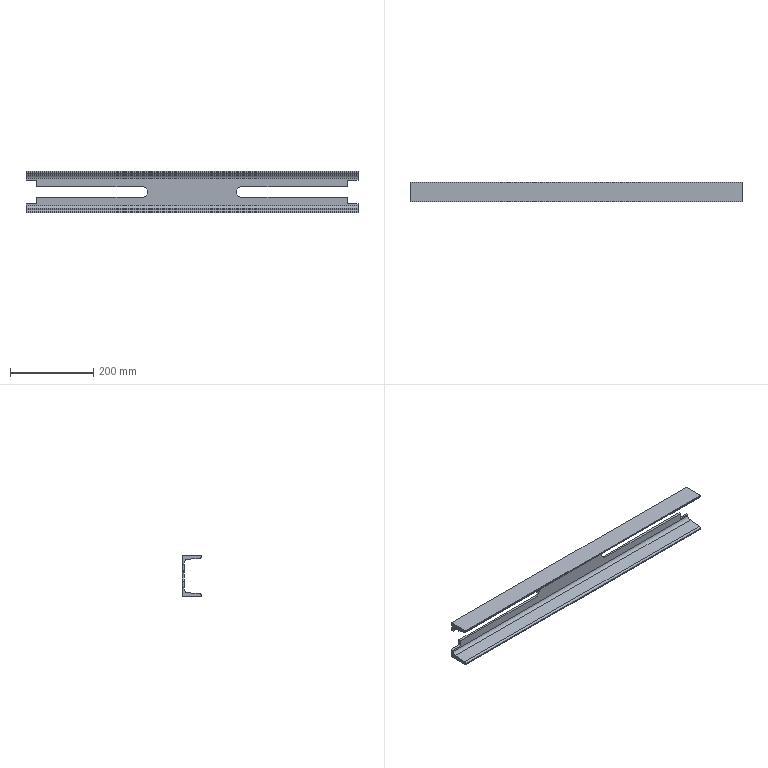Part | SolidWorks | features ICE 2, MirrorPattern 1, WeldMemberFeat 1, WeldmentFeature 1 | 1 solid | 30 faces | box 800 x 48 x 100 mm | volume 931477 mm3 | plane 24 | cylinder 6 | commonest cylinder face diameters 8.5 x2 17 x2 26 x2
STEP:
#1=CARTESIAN_POINT('',(400.,0.,78.));
#2=VERTEX_POINT('',#1);
#3=CARTESIAN_POINT('',(375.,0.,78.));
#4=VERTEX_POINT('',#3);
#5=CARTESIAN_POINT('',(400.,0.,78.));
#6=DIRECTION('',(-1.,0.,0.));
#7=VECTOR('',#6,1000.);
#8=LINE('',#5,#7);
#9=EDGE_CURVE('',#2,#4,#8,.T.);
#10=ORIENTED_EDGE('',*,*,#9,.T.);
#11=CARTESIAN_POINT('',(375.,0.,63.));
#12=VERTEX_POINT('',#11);
#13=CARTESIAN_POINT('',(375.,0.,78.));
#14=DIRECTION('',(0.,0.,-1.));
#15=VECTOR('',#14,1000.);
#16=LINE('',#13,#15);
#17=EDGE_CURVE('',#4,#12,#16,.T.);
#18=ORIENTED_EDGE('',*,*,#17,.T.);
#19=CARTESIAN_POINT('',(120.,0.,63.));
#20=VERTEX_POINT('',#19);
#21=CARTESIAN_POINT('',(680.,0.,63.));
#22=DIRECTION('',(-1.,0.,0.));
#23=VECTOR('',#22,1000.);
#24=LINE('',#21,#23);
#25=EDGE_CURVE('',#12,#20,#24,.T.);
#26=ORIENTED_EDGE('',*,*,#25,.T.);
#27=CARTESIAN_POINT('',(120.,0.,37.));
#28=VERTEX_POINT('',#27);
#29=CARTESIAN_POINT('',(120.,0.,50.));
#30=DIRECTION('',(0.,-1.,0.));
#31=DIRECTION('',(0.,0.,1.));
#32=AXIS2_PLACEMENT_3D('',#29,#30,#31);
#33=CIRCLE('',#32,13.);
#34=EDGE_CURVE('',#20,#28,#33,.T.);
#35=ORIENTED_EDGE('',*,*,#34,.T.);
#36=CARTESIAN_POINT('',(375.,0.,37.));
#37=VERTEX_POINT('',#36);
#38=CARTESIAN_POINT('',(680.,0.,37.));
#39=DIRECTION('',(1.,0.,0.));
#40=VECTOR('',#39,1000.);
#41=LINE('',#38,#40);
#42=EDGE_CURVE('',#28,#37,#41,.T.);
#43=ORIENTED_EDGE('',*,*,#42,.T.);
#44=CARTESIAN_POINT('',(375.,0.,22.));
#45=VERTEX_POINT('',#44);
#46=CARTESIAN_POINT('',(375.,0.,22.));
#47=DIRECTION('',(0.,0.,-1.));
#48=VECTOR('',#47,1000.);
#49=LINE('',#46,#48);
#50=EDGE_CURVE('',#37,#45,#49,.T.);
#51=ORIENTED_EDGE('',*,*,#50,.T.);
#52=CARTESIAN_POINT('',(400.,0.,22.));
#53=VERTEX_POINT('',#52);
#54=CARTESIAN_POINT('',(400.,0.,22.));
#55=DIRECTION('',(1.,0.,0.));
#56=VECTOR('',#55,1000.);
#57=LINE('',#54,#56);
#58=EDGE_CURVE('',#45,#53,#57,.T.);
#59=ORIENTED_EDGE('',*,*,#58,.T.);
#60=CARTESIAN_POINT('',(400.,0.,0.));
#61=VERTEX_POINT('',#60);
#62=CARTESIAN_POINT('',(400.,0.,100.));
#63=DIRECTION('',(0.,0.,-1.));
#64=VECTOR('',#63,1000.);
#65=LINE('',#62,#64);
#66=EDGE_CURVE('',#53,#61,#65,.T.);
#67=ORIENTED_EDGE('',*,*,#66,.T.);
#68=CARTESIAN_POINT('',(-400.,0.,0.));
#69=VERTEX_POINT('',#68);
#70=CARTESIAN_POINT('',(-400.,0.,0.));
#71=DIRECTION('',(1.,0.,0.));
#72=VECTOR('',#71,1000.);
#73=LINE('',#70,#72);
#74=EDGE_CURVE('',#69,#61,#73,.T.);
#75=ORIENTED_EDGE('',*,*,#74,.F.);
#76=CARTESIAN_POINT('',(-400.,0.,22.));
#77=VERTEX_POINT('',#76);
#78=CARTESIAN_POINT('',(-400.,0.,100.));
#79=DIRECTION('',(0.,0.,-1.));
#80=VECTOR('',#79,1000.);
#81=LINE('',#78,#80);
#82=EDGE_CURVE('',#77,#69,#81,.T.);
#83=ORIENTED_EDGE('',*,*,#82,.F.);
#84=CARTESIAN_POINT('',(-375.,0.,22.));
#85=VERTEX_POINT('',#84);
#86=CARTESIAN_POINT('',(-400.,0.,22.));
#87=DIRECTION('',(-1.,0.,0.));
#88=VECTOR('',#87,1000.);
#89=LINE('',#86,#88);
#90=EDGE_CURVE('',#85,#77,#89,.T.);
#91=ORIENTED_EDGE('',*,*,#90,.F.);
#92=CARTESIAN_POINT('',(-375.,0.,37.));
#93=VERTEX_POINT('',#92);
#94=CARTESIAN_POINT('',(-375.,0.,22.));
#95=DIRECTION('',(0.,0.,-1.));
#96=VECTOR('',#95,1000.);
#97=LINE('',#94,#96);
#98=EDGE_CURVE('',#93,#85,#97,.T.);
#99=ORIENTED_EDGE('',*,*,#98,.F.);
#100=CARTESIAN_POINT('',(-120.,0.,37.));
#101=VERTEX_POINT('',#100);
#102=CARTESIAN_POINT('',(-680.,0.,37.));
#103=DIRECTION('',(-1.,0.,0.));
#104=VECTOR('',#103,1000.);
#105=LINE('',#102,#104);
#106=EDGE_CURVE('',#101,#93,#105,.T.);
#107=ORIENTED_EDGE('',*,*,#106,.F.);
#108=CARTESIAN_POINT('',(-120.,0.,63.));
#109=VERTEX_POINT('',#108);
#110=CARTESIAN_POINT('',(-120.,0.,50.));
#111=DIRECTION('',(0.,1.,0.));
#112=DIRECTION('',(0.,0.,1.));
#113=AXIS2_PLACEMENT_3D('',#110,#111,#112);
#114=CIRCLE('',#113,13.);
#115=EDGE_CURVE('',#109,#101,#114,.T.);
#116=ORIENTED_EDGE('',*,*,#115,.F.);
#117=CARTESIAN_POINT('',(-375.,0.,63.));
#118=VERTEX_POINT('',#117);
#119=CARTESIAN_POINT('',(-680.,0.,63.));
#120=DIRECTION('',(1.,0.,0.));
#121=VECTOR('',#120,1000.);
#122=LINE('',#119,#121);
#123=EDGE_CURVE('',#118,#109,#122,.T.);
#124=ORIENTED_EDGE('',*,*,#123,.F.);
#125=CARTESIAN_POINT('',(-375.,0.,78.));
#126=VERTEX_POINT('',#125);
#127=CARTESIAN_POINT('',(-375.,0.,78.));
#128=DIRECTION('',(0.,0.,-1.));
#129=VECTOR('',#128,1000.);
#130=LINE('',#127,#129);
#131=EDGE_CURVE('',#126,#118,#130,.T.);
#132=ORIENTED_EDGE('',*,*,#131,.F.);
#133=CARTESIAN_POINT('',(-400.,0.,78.));
#134=VERTEX_POINT('',#133);
#135=CARTESIAN_POINT('',(-400.,0.,78.));
#136=DIRECTION('',(1.,0.,0.));
#137=VECTOR('',#136,1000.);
#138=LINE('',#135,#137);
#139=EDGE_CURVE('',#134,#126,#138,.T.);
#140=ORIENTED_EDGE('',*,*,#139,.F.);
#141=CARTESIAN_POINT('',(-400.,0.,100.));
#142=VERTEX_POINT('',#141);
#143=CARTESIAN_POINT('',(-400.,0.,100.));
#144=DIRECTION('',(0.,0.,-1.));
#145=VECTOR('',#144,1000.);
#146=LINE('',#143,#145);
#147=EDGE_CURVE('',#142,#134,#146,.T.);
#148=ORIENTED_EDGE('',*,*,#147,.F.);
#149=CARTESIAN_POINT('',(400.,0.,100.));
#150=VERTEX_POINT('',#149);
#151=CARTESIAN_POINT('',(-400.,0.,100.));
#152=DIRECTION('',(1.,0.,0.));
#153=VECTOR('',#152,1000.);
#154=LINE('',#151,#153);
#155=EDGE_CURVE('',#142,#150,#154,.T.);
#156=ORIENTED_EDGE('',*,*,#155,.T.);
#157=CARTESIAN_POINT('',(400.,0.,100.));
#158=DIRECTION('',(0.,0.,-1.));
#159=VECTOR('',#158,1000.);
#160=LINE('',#157,#159);
#161=EDGE_CURVE('',#150,#2,#160,.T.);
#162=ORIENTED_EDGE('',*,*,#161,.T.);
#163=EDGE_LOOP('',(#10,#18,#26,#35,#43,#51,#59,#67,#75,#83,#91,#99,#107,#116,#124,#132,#140,#148,#156,#162));
#164=FACE_OUTER_BOUND('',#163,.T.);
#165=CARTESIAN_POINT('',(-400.,0.,100.));
#166=DIRECTION('',(0.,-1.,0.));
#167=DIRECTION('',(1.,0.,0.));
#168=AXIS2_PLACEMENT_3D('',#165,#166,#167);
#169=PLANE('',#168);
#170=ADVANCED_FACE('',(#164),#169,.F.);
#171=CARTESIAN_POINT('',(400.,-5.3,78.));
#172=VERTEX_POINT('',#171);
#173=CARTESIAN_POINT('',(375.,-5.3,78.));
#174=VERTEX_POINT('',#173);
#175=CARTESIAN_POINT('',(-400.,-5.3,78.));
#176=DIRECTION('',(-1.,0.,0.));
#177=VECTOR('',#176,1000.);
#178=LINE('',#175,#177);
#179=EDGE_CURVE('',#172,#174,#178,.T.);
#180=ORIENTED_EDGE('',*,*,#179,.F.);
#181=CARTESIAN_POINT('',(400.,-5.3,81.673));
#182=VERTEX_POINT('',#181);
#183=CARTESIAN_POINT('',(400.,-5.3,81.673));
#184=DIRECTION('',(0.,0.,1.));
#185=VECTOR('',#184,1000.);
#186=LINE('',#183,#185);
#187=EDGE_CURVE('',#172,#182,#186,.T.);
#188=ORIENTED_EDGE('',*,*,#187,.T.);
#189=CARTESIAN_POINT('',(-400.,-5.3,81.673));
#190=VERTEX_POINT('',#189);
#191=CARTESIAN_POINT('',(-400.,-5.3,81.673));
#192=DIRECTION('',(1.,0.,0.));
#193=VECTOR('',#192,1000.);
#194=LINE('',#191,#193);
#195=EDGE_CURVE('',#190,#182,#194,.T.);
#196=ORIENTED_EDGE('',*,*,#195,.F.);
#197=CARTESIAN_POINT('',(-400.,-5.3,78.));
#198=VERTEX_POINT('',#197);
#199=CARTESIAN_POINT('',(-400.,-5.3,81.673));
#200=DIRECTION('',(0.,0.,1.));
#201=VECTOR('',#200,1000.);
#202=LINE('',#199,#201);
#203=EDGE_CURVE('',#198,#190,#202,.T.);
#204=ORIENTED_EDGE('',*,*,#203,.F.);
#205=CARTESIAN_POINT('',(-375.,-5.3,78.));
#206=VERTEX_POINT('',#205);
#207=CARTESIAN_POINT('',(-400.,-5.3,78.));
#208=DIRECTION('',(1.,0.,0.));
#209=VECTOR('',#208,1000.);
#210=LINE('',#207,#209);
#211=EDGE_CURVE('',#198,#206,#210,.T.);
#212=ORIENTED_EDGE('',*,*,#211,.T.);
#213=CARTESIAN_POINT('',(-375.,-5.3,63.));
#214=VERTEX_POINT('',#213);
#215=CARTESIAN_POINT('',(-375.,-5.3,81.673));
#216=DIRECTION('',(0.,0.,-1.));
#217=VECTOR('',#216,1000.);
#218=LINE('',#215,#217);
#219=EDGE_CURVE('',#206,#214,#218,.T.);
#220=ORIENTED_EDGE('',*,*,#219,.T.);
#221=CARTESIAN_POINT('',(-120.,-5.3,63.));
#222=VERTEX_POINT('',#221);
#223=CARTESIAN_POINT('',(-400.,-5.3,63.));
#224=DIRECTION('',(1.,0.,0.));
#225=VECTOR('',#224,1000.);
#226=LINE('',#223,#225);
#227=EDGE_CURVE('',#214,#222,#226,.T.);
#228=ORIENTED_EDGE('',*,*,#227,.T.);
#229=CARTESIAN_POINT('',(-120.,-5.3,37.));
#230=VERTEX_POINT('',#229);
#231=CARTESIAN_POINT('',(-120.,-5.3,50.));
#232=DIRECTION('',(0.,1.,0.));
#233=DIRECTION('',(-1.,0.,0.));
#234=AXIS2_PLACEMENT_3D('',#231,#232,#233);
#235=CIRCLE('',#234,13.);
#236=EDGE_CURVE('',#222,#230,#235,.T.);
#237=ORIENTED_EDGE('',*,*,#236,.T.);
#238=CARTESIAN_POINT('',(-375.,-5.3,37.));
#239=VERTEX_POINT('',#238);
#240=CARTESIAN_POINT('',(-400.,-5.3,37.));
#241=DIRECTION('',(-1.,0.,0.));
#242=VECTOR('',#241,1000.);
#243=LINE('',#240,#242);
#244=EDGE_CURVE('',#230,#239,#243,.T.);
#245=ORIENTED_EDGE('',*,*,#244,.T.);
#246=CARTESIAN_POINT('',(-375.,-5.3,22.));
#247=VERTEX_POINT('',#246);
#248=CARTESIAN_POINT('',(-375.,-5.3,81.673));
#249=DIRECTION('',(0.,0.,-1.));
#250=VECTOR('',#249,1000.);
#251=LINE('',#248,#250);
#252=EDGE_CURVE('',#239,#247,#251,.T.);
#253=ORIENTED_EDGE('',*,*,#252,.T.);
#254=CARTESIAN_POINT('',(-400.,-5.3,22.));
#255=VERTEX_POINT('',#254);
#256=CARTESIAN_POINT('',(-400.,-5.3,22.));
#257=DIRECTION('',(-1.,0.,0.));
#258=VECTOR('',#257,1000.);
#259=LINE('',#256,#258);
#260=EDGE_CURVE('',#247,#255,#259,.T.);
#261=ORIENTED_EDGE('',*,*,#260,.T.);
#262=CARTESIAN_POINT('',(-400.,-5.3,18.327));
#263=VERTEX_POINT('',#262);
#264=CARTESIAN_POINT('',(-400.,-5.3,81.673));
#265=DIRECTION('',(0.,0.,1.));
#266=VECTOR('',#265,1000.);
#267=LINE('',#264,#266);
#268=EDGE_CURVE('',#263,#255,#267,.T.);
#269=ORIENTED_EDGE('',*,*,#268,.F.);
#270=CARTESIAN_POINT('',(400.,-5.3,18.327));
#271=VERTEX_POINT('',#270);
#272=CARTESIAN_POINT('',(-400.,-5.3,18.327));
#273=DIRECTION('',(1.,0.,0.));
#274=VECTOR('',#273,1000.);
#275=LINE('',#272,#274);
#276=EDGE_CURVE('',#263,#271,#275,.T.);
#277=ORIENTED_EDGE('',*,*,#276,.T.);
#278=CARTESIAN_POINT('',(400.,-5.3,22.));
#279=VERTEX_POINT('',#278);
#280=CARTESIAN_POINT('',(400.,-5.3,81.673));
#281=DIRECTION('',(0.,0.,1.));
#282=VECTOR('',#281,1000.);
#283=LINE('',#280,#282);
#284=EDGE_CURVE('',#271,#279,#283,.T.);
#285=ORIENTED_EDGE('',*,*,#284,.T.);
#286=CARTESIAN_POINT('',(375.,-5.3,22.));
#287=VERTEX_POINT('',#286);
#288=CARTESIAN_POINT('',(-400.,-5.3,22.));
#289=DIRECTION('',(1.,0.,0.));
#290=VECTOR('',#289,1000.);
#291=LINE('',#288,#290);
#292=EDGE_CURVE('',#287,#279,#291,.T.);
#293=ORIENTED_EDGE('',*,*,#292,.F.);
#294=CARTESIAN_POINT('',(375.,-5.3,37.));
#295=VERTEX_POINT('',#294);
#296=CARTESIAN_POINT('',(375.,-5.3,81.673));
#297=DIRECTION('',(0.,0.,-1.));
#298=VECTOR('',#297,1000.);
#299=LINE('',#296,#298);
#300=EDGE_CURVE('',#295,#287,#299,.T.);
#301=ORIENTED_EDGE('',*,*,#300,.F.);
#302=CARTESIAN_POINT('',(120.,-5.3,37.));
#303=VERTEX_POINT('',#302);
#304=CARTESIAN_POINT('',(-400.,-5.3,37.));
#305=DIRECTION('',(1.,0.,0.));
#306=VECTOR('',#305,1000.);
#307=LINE('',#304,#306);
#308=EDGE_CURVE('',#303,#295,#307,.T.);
#309=ORIENTED_EDGE('',*,*,#308,.F.);
#310=CARTESIAN_POINT('',(120.,-5.3,63.));
#311=VERTEX_POINT('',#310);
#312=CARTESIAN_POINT('',(120.,-5.3,50.));
#313=DIRECTION('',(0.,-1.,0.));
#314=DIRECTION('',(-1.,0.,0.));
#315=AXIS2_PLACEMENT_3D('',#312,#313,#314);
#316=CIRCLE('',#315,13.);
#317=EDGE_CURVE('',#311,#303,#316,.T.);
#318=ORIENTED_EDGE('',*,*,#317,.F.);
#319=CARTESIAN_POINT('',(375.,-5.3,63.));
#320=VERTEX_POINT('',#319);
#321=CARTESIAN_POINT('',(-400.,-5.3,63.));
#322=DIRECTION('',(-1.,0.,0.));
#323=VECTOR('',#322,1000.);
#324=LINE('',#321,#323);
#325=EDGE_CURVE('',#320,#311,#324,.T.);
#326=ORIENTED_EDGE('',*,*,#325,.F.);
#327=CARTESIAN_POINT('',(375.,-5.3,81.673));
#328=DIRECTION('',(0.,0.,-1.));
#329=VECTOR('',#328,1000.);
#330=LINE('',#327,#329);
#331=EDGE_CURVE('',#174,#320,#330,.T.);
#332=ORIENTED_EDGE('',*,*,#331,.F.);
#333=EDGE_LOOP('',(#180,#188,#196,#204,#212,#220,#228,#237,#245,#253,#261,#269,#277,#285,#293,#301,#309,#318,#326,#332));
#334=FACE_OUTER_BOUND('',#333,.T.);
#335=CARTESIAN_POINT('',(-400.,-5.3,81.673));
#336=DIRECTION('',(0.,1.,0.));
#337=DIRECTION('',(-1.,0.,0.));
#338=AXIS2_PLACEMENT_3D('',#335,#336,#337);
#339=PLANE('',#338);
#340=ADVANCED_FACE('',(#334),#339,.F.);
#341=CARTESIAN_POINT('',(400.,-10.,78.));
#342=DIRECTION('',(0.,1.,0.));
#343=VECTOR('',#342,1000.);
#344=LINE('',#341,#343);
#345=EDGE_CURVE('',#172,#2,#344,.T.);
#346=ORIENTED_EDGE('',*,*,#345,.T.);
#347=ORIENTED_EDGE('',*,*,#161,.F.);
#348=CARTESIAN_POINT('',(400.,-48.,100.));
#349=VERTEX_POINT('',#348);
#350=CARTESIAN_POINT('',(400.,-48.,100.));
#351=DIRECTION('',(0.,1.,0.));
#352=VECTOR('',#351,1000.);
#353=LINE('',#350,#352);
#354=EDGE_CURVE('',#349,#150,#353,.T.);
#355=ORIENTED_EDGE('',*,*,#354,.F.);
#356=CARTESIAN_POINT('',(400.,-48.,97.481));
#357=VERTEX_POINT('',#356);
#358=CARTESIAN_POINT('',(400.,-48.,100.));
#359=DIRECTION('',(0.,0.,1.));
#360=VECTOR('',#359,1000.);
#361=LINE('',#358,#360);
#362=EDGE_CURVE('',#357,#349,#361,.T.);
#363=ORIENTED_EDGE('',*,*,#362,.F.);
#364=CARTESIAN_POINT('',(400.,-44.173,93.252));
#365=VERTEX_POINT('',#364);
#366=CARTESIAN_POINT('',(400.,-43.75,97.481));
#367=DIRECTION('',(-1.,0.,0.));
#368=DIRECTION('',(0.,-1.,0.));
#369=AXIS2_PLACEMENT_3D('',#366,#367,#368);
#370=CIRCLE('',#369,4.25);
#371=EDGE_CURVE('',#365,#357,#370,.T.);
#372=ORIENTED_EDGE('',*,*,#371,.F.);
#373=CARTESIAN_POINT('',(400.,-12.954,90.13));
#374=VERTEX_POINT('',#373);
#375=CARTESIAN_POINT('',(400.,-12.954,90.13));
#376=DIRECTION('',(0.,-0.995,0.0995));
#377=VECTOR('',#376,1000.);
#378=LINE('',#375,#377);
#379=EDGE_CURVE('',#374,#365,#378,.T.);
#380=ORIENTED_EDGE('',*,*,#379,.F.);
#381=CARTESIAN_POINT('',(400.,-13.8,81.673));
#382=DIRECTION('',(1.,0.,0.));
#383=DIRECTION('',(0.,1.,0.));
#384=AXIS2_PLACEMENT_3D('',#381,#382,#383);
#385=CIRCLE('',#384,8.5);
#386=EDGE_CURVE('',#182,#374,#385,.T.);
#387=ORIENTED_EDGE('',*,*,#386,.F.);
#388=ORIENTED_EDGE('',*,*,#187,.F.);
#389=EDGE_LOOP('',(#346,#347,#355,#363,#372,#380,#387,#388));
#390=FACE_OUTER_BOUND('',#389,.T.);
#391=CARTESIAN_POINT('',(400.,-43.75,97.481));
#392=DIRECTION('',(-1.,0.,0.));
#393=DIRECTION('',(0.,-1.,0.));
#394=AXIS2_PLACEMENT_3D('',#391,#392,#393);
#395=PLANE('',#394);
#396=ADVANCED_FACE('',(#390),#395,.F.);
#397=ORIENTED_EDGE('',*,*,#25,.F.);
#398=CARTESIAN_POINT('',(375.,-10.,63.));
#399=DIRECTION('',(0.,-1.,0.));
#400=VECTOR('',#399,1000.);
#401=LINE('',#398,#400);
#402=EDGE_CURVE('',#12,#320,#401,.T.);
#403=ORIENTED_EDGE('',*,*,#402,.T.);
#404=ORIENTED_EDGE('',*,*,#325,.T.);
#405=CARTESIAN_POINT('',(120.,-10.,63.));
#406=DIRECTION('',(0.,1.,0.));
#407=VECTOR('',#406,1000.);
#408=LINE('',#405,#407);
#409=EDGE_CURVE('',#311,#20,#408,.T.);
#410=ORIENTED_EDGE('',*,*,#409,.T.);
#411=EDGE_LOOP('',(#397,#403,#404,#410));
#412=FACE_OUTER_BOUND('',#411,.T.);
#413=CARTESIAN_POINT('',(680.,-10.,63.));
#414=DIRECTION('',(0.,0.,-1.));
#415=DIRECTION('',(0.,1.,0.));
#416=AXIS2_PLACEMENT_3D('',#413,#414,#415);
#417=PLANE('',#416);
#418=ADVANCED_FACE('',(#412),#417,.T.);
#419=CARTESIAN_POINT('',(400.,-10.,22.));
#420=DIRECTION('',(0.,1.,0.));
#421=VECTOR('',#420,1000.);
#422=LINE('',#419,#421);
#423=EDGE_CURVE('',#279,#53,#422,.T.);
#424=ORIENTED_EDGE('',*,*,#423,.F.);
#425=ORIENTED_EDGE('',*,*,#284,.F.);
#426=CARTESIAN_POINT('',(400.,-12.954,9.87));
#427=VERTEX_POINT('',#426);
#428=CARTESIAN_POINT('',(400.,-13.8,18.327));
#429=DIRECTION('',(1.,0.,0.));
#430=DIRECTION('',(0.,-1.,0.));
#431=AXIS2_PLACEMENT_3D('',#428,#429,#430);
#432=CIRCLE('',#431,8.5);
#433=EDGE_CURVE('',#427,#271,#432,.T.);
#434=ORIENTED_EDGE('',*,*,#433,.F.);
#435=CARTESIAN_POINT('',(400.,-44.173,6.748));
#436=VERTEX_POINT('',#435);
#437=CARTESIAN_POINT('',(400.,-12.954,9.87));
#438=DIRECTION('',(0.,0.995,0.0995));
#439=VECTOR('',#438,1000.);
#440=LINE('',#437,#439);
#441=EDGE_CURVE('',#436,#427,#440,.T.);
#442=ORIENTED_EDGE('',*,*,#441,.F.);
#443=CARTESIAN_POINT('',(400.,-48.,2.519));
#444=VERTEX_POINT('',#443);
#445=CARTESIAN_POINT('',(400.,-43.75,2.519));
#446=DIRECTION('',(-1.,0.,0.));
#447=DIRECTION('',(0.,1.,0.));
#448=AXIS2_PLACEMENT_3D('',#445,#446,#447);
#449=CIRCLE('',#448,4.25);
#450=EDGE_CURVE('',#444,#436,#449,.T.);
#451=ORIENTED_EDGE('',*,*,#450,.F.);
#452=CARTESIAN_POINT('',(400.,-48.,0.));
#453=VERTEX_POINT('',#452);
#454=CARTESIAN_POINT('',(400.,-48.,0.));
#455=DIRECTION('',(0.,0.,1.));
#456=VECTOR('',#455,1000.);
#457=LINE('',#454,#456);
#458=EDGE_CURVE('',#453,#444,#457,.T.);
#459=ORIENTED_EDGE('',*,*,#458,.F.);
#460=CARTESIAN_POINT('',(400.,-48.,0.));
#461=DIRECTION('',(0.,-1.,0.));
#462=VECTOR('',#461,1000.);
#463=LINE('',#460,#462);
#464=EDGE_CURVE('',#61,#453,#463,.T.);
#465=ORIENTED_EDGE('',*,*,#464,.F.);
#466=ORIENTED_EDGE('',*,*,#66,.F.);
#467=EDGE_LOOP('',(#424,#425,#434,#442,#451,#459,#465,#466));
#468=FACE_OUTER_BOUND('',#467,.T.);
#469=CARTESIAN_POINT('',(400.,-43.75,97.481));
#470=DIRECTION('',(-1.,0.,0.));
#471=DIRECTION('',(0.,-1.,0.));
#472=AXIS2_PLACEMENT_3D('',#469,#470,#471);
#473=PLANE('',#472);
#474=ADVANCED_FACE('',(#468),#473,.F.);
#475=ORIENTED_EDGE('',*,*,#308,.T.);
#476=CARTESIAN_POINT('',(375.,-10.,37.));
#477=DIRECTION('',(0.,1.,0.));
#478=VECTOR('',#477,1000.);
#479=LINE('',#476,#478);
#480=EDGE_CURVE('',#295,#37,#479,.T.);
#481=ORIENTED_EDGE('',*,*,#480,.T.);
#482=ORIENTED_EDGE('',*,*,#42,.F.);
#483=CARTESIAN_POINT('',(120.,-10.,37.));
#484=DIRECTION('',(0.,1.,0.));
#485=VECTOR('',#484,1000.);
#486=LINE('',#483,#485);
#487=EDGE_CURVE('',#303,#28,#486,.T.);
#488=ORIENTED_EDGE('',*,*,#487,.F.);
#489=EDGE_LOOP('',(#475,#481,#482,#488));
#490=FACE_OUTER_BOUND('',#489,.T.);
#491=CARTESIAN_POINT('',(680.,-10.,37.));
#492=DIRECTION('',(0.,0.,1.));
#493=DIRECTION('',(0.,-1.,0.));
#494=AXIS2_PLACEMENT_3D('',#491,#492,#493);
#495=PLANE('',#494);
#496=ADVANCED_FACE('',(#490),#495,.T.);
#497=CARTESIAN_POINT('',(-400.,-10.,22.));
#498=DIRECTION('',(0.,1.,0.));
#499=VECTOR('',#498,1000.);
#500=LINE('',#497,#499);
#501=EDGE_CURVE('',#255,#77,#500,.T.);
#502=ORIENTED_EDGE('',*,*,#501,.T.);
#503=ORIENTED_EDGE('',*,*,#82,.T.);
#504=CARTESIAN_POINT('',(-400.,-48.,0.));
#505=VERTEX_POINT('',#504);
#506=CARTESIAN_POINT('',(-400.,-48.,0.));
#507=DIRECTION('',(0.,-1.,0.));
#508=VECTOR('',#507,1000.);
#509=LINE('',#506,#508);
#510=EDGE_CURVE('',#69,#505,#509,.T.);
#511=ORIENTED_EDGE('',*,*,#510,.T.);
#512=CARTESIAN_POINT('',(-400.,-48.,2.519));
#513=VERTEX_POINT('',#512);
#514=CARTESIAN_POINT('',(-400.,-48.,0.));
#515=DIRECTION('',(0.,0.,1.));
#516=VECTOR('',#515,1000.);
#517=LINE('',#514,#516);
#518=EDGE_CURVE('',#505,#513,#517,.T.);
#519=ORIENTED_EDGE('',*,*,#518,.T.);
#520=CARTESIAN_POINT('',(-400.,-44.173,6.748));
#521=VERTEX_POINT('',#520);
#522=CARTESIAN_POINT('',(-400.,-43.75,2.519));
#523=DIRECTION('',(-1.,0.,0.));
#524=DIRECTION('',(0.,1.,0.));
#525=AXIS2_PLACEMENT_3D('',#522,#523,#524);
#526=CIRCLE('',#525,4.25);
#527=EDGE_CURVE('',#513,#521,#526,.T.);
#528=ORIENTED_EDGE('',*,*,#527,.T.);
#529=CARTESIAN_POINT('',(-400.,-12.954,9.87));
#530=VERTEX_POINT('',#529);
#531=CARTESIAN_POINT('',(-400.,-12.954,9.87));
#532=DIRECTION('',(0.,0.995,0.0995));
#533=VECTOR('',#532,1000.);
#534=LINE('',#531,#533);
#535=EDGE_CURVE('',#521,#530,#534,.T.);
#536=ORIENTED_EDGE('',*,*,#535,.T.);
#537=CARTESIAN_POINT('',(-400.,-13.8,18.327));
#538=DIRECTION('',(1.,0.,0.));
#539=DIRECTION('',(0.,-1.,0.));
#540=AXIS2_PLACEMENT_3D('',#537,#538,#539);
#541=CIRCLE('',#540,8.5);
#542=EDGE_CURVE('',#530,#263,#541,.T.);
#543=ORIENTED_EDGE('',*,*,#542,.T.);
#544=ORIENTED_EDGE('',*,*,#268,.T.);
#545=EDGE_LOOP('',(#502,#503,#511,#519,#528,#536,#543,#544));
#546=FACE_OUTER_BOUND('',#545,.T.);
#547=CARTESIAN_POINT('',(-400.,-43.75,97.481));
#548=DIRECTION('',(-1.,0.,0.));
#549=DIRECTION('',(0.,-1.,0.));
#550=AXIS2_PLACEMENT_3D('',#547,#548,#549);
#551=PLANE('',#550);
#552=ADVANCED_FACE('',(#546),#551,.T.);
#553=ORIENTED_EDGE('',*,*,#371,.T.);
#554=CARTESIAN_POINT('',(-400.,-48.,97.481));
#555=VERTEX_POINT('',#554);
#556=CARTESIAN_POINT('',(-400.,-48.,97.481));
#557=DIRECTION('',(1.,0.,0.));
#558=VECTOR('',#557,1000.);
#559=LINE('',#556,#558);
#560=EDGE_CURVE('',#555,#357,#559,.T.);
#561=ORIENTED_EDGE('',*,*,#560,.F.);
#562=CARTESIAN_POINT('',(-400.,-44.173,93.252));
#563=VERTEX_POINT('',#562);
#564=CARTESIAN_POINT('',(-400.,-43.75,97.481));
#565=DIRECTION('',(-1.,0.,0.));
#566=DIRECTION('',(0.,-1.,0.));
#567=AXIS2_PLACEMENT_3D('',#564,#565,#566);
#568=CIRCLE('',#567,4.25);
#569=EDGE_CURVE('',#563,#555,#568,.T.);
#570=ORIENTED_EDGE('',*,*,#569,.F.);
#571=CARTESIAN_POINT('',(-400.,-44.173,93.252));
#572=DIRECTION('',(1.,0.,0.));
#573=VECTOR('',#572,1000.);
#574=LINE('',#571,#573);
#575=EDGE_CURVE('',#563,#365,#574,.T.);
#576=ORIENTED_EDGE('',*,*,#575,.T.);
#577=EDGE_LOOP('',(#553,#561,#570,#576));
#578=FACE_OUTER_BOUND('',#577,.T.);
#579=CARTESIAN_POINT('',(-400.,-43.75,97.481));
#580=DIRECTION('',(1.,0.,0.));
#581=DIRECTION('',(0.,1.,0.));
#582=AXIS2_PLACEMENT_3D('',#579,#580,#581);
#583=CYLINDRICAL_SURFACE('',#582,4.25);
#584=ADVANCED_FACE('',(#578),#583,.T.);
#585=ORIENTED_EDGE('',*,*,#362,.T.);
#586=CARTESIAN_POINT('',(-400.,-48.,100.));
#587=VERTEX_POINT('',#586);
#588=CARTESIAN_POINT('',(-400.,-48.,100.));
#589=DIRECTION('',(1.,0.,0.));
#590=VECTOR('',#589,1000.);
#591=LINE('',#588,#590);
#592=EDGE_CURVE('',#587,#349,#591,.T.);
#593=ORIENTED_EDGE('',*,*,#592,.F.);
#594=CARTESIAN_POINT('',(-400.,-48.,100.));
#595=DIRECTION('',(0.,0.,1.));
#596=VECTOR('',#595,1000.);
#597=LINE('',#594,#596);
#598=EDGE_CURVE('',#555,#587,#597,.T.);
#599=ORIENTED_EDGE('',*,*,#598,.F.);
#600=ORIENTED_EDGE('',*,*,#560,.T.);
#601=EDGE_LOOP('',(#585,#593,#599,#600));
#602=FACE_OUTER_BOUND('',#601,.T.);
#603=CARTESIAN_POINT('',(-400.,-48.,100.));
#604=DIRECTION('',(0.,1.,0.));
#605=DIRECTION('',(0.,0.,1.));
#606=AXIS2_PLACEMENT_3D('',#603,#604,#605);
#607=PLANE('',#606);
#608=ADVANCED_FACE('',(#602),#607,.F.);
#609=ORIENTED_EDGE('',*,*,#354,.T.);
#610=ORIENTED_EDGE('',*,*,#155,.F.);
#611=CARTESIAN_POINT('',(-400.,-48.,100.));
#612=DIRECTION('',(0.,1.,0.));
#613=VECTOR('',#612,1000.);
#614=LINE('',#611,#613);
#615=EDGE_CURVE('',#587,#142,#614,.T.);
#616=ORIENTED_EDGE('',*,*,#615,.F.);
#617=ORIENTED_EDGE('',*,*,#592,.T.);
#618=EDGE_LOOP('',(#609,#610,#616,#617));
#619=FACE_OUTER_BOUND('',#618,.T.);
#620=CARTESIAN_POINT('',(-400.,-48.,100.));
#621=DIRECTION('',(0.,0.,-1.));
#622=DIRECTION('',(0.,1.,0.));
#623=AXIS2_PLACEMENT_3D('',#620,#621,#622);
#624=PLANE('',#623);
#625=ADVANCED_FACE('',(#619),#624,.F.);
#626=ORIENTED_EDGE('',*,*,#464,.T.);
#627=CARTESIAN_POINT('',(-400.,-48.,0.));
#628=DIRECTION('',(1.,0.,0.));
#629=VECTOR('',#628,1000.);
#630=LINE('',#627,#629);
#631=EDGE_CURVE('',#505,#453,#630,.T.);
#632=ORIENTED_EDGE('',*,*,#631,.F.);
#633=ORIENTED_EDGE('',*,*,#510,.F.);
#634=ORIENTED_EDGE('',*,*,#74,.T.);
#635=EDGE_LOOP('',(#626,#632,#633,#634));
#636=FACE_OUTER_BOUND('',#635,.T.);
#637=CARTESIAN_POINT('',(-400.,-48.,0.));
#638=DIRECTION('',(0.,0.,1.));
#639=DIRECTION('',(0.,-1.,0.));
#640=AXIS2_PLACEMENT_3D('',#637,#638,#639);
#641=PLANE('',#640);
#642=ADVANCED_FACE('',(#636),#641,.F.);
#643=ORIENTED_EDGE('',*,*,#458,.T.);
#644=CARTESIAN_POINT('',(-400.,-48.,2.519));
#645=DIRECTION('',(1.,0.,0.));
#646=VECTOR('',#645,1000.);
#647=LINE('',#644,#646);
#648=EDGE_CURVE('',#513,#444,#647,.T.);
#649=ORIENTED_EDGE('',*,*,#648,.F.);
#650=ORIENTED_EDGE('',*,*,#518,.F.);
#651=ORIENTED_EDGE('',*,*,#631,.T.);
#652=EDGE_LOOP('',(#643,#649,#650,#651));
#653=FACE_OUTER_BOUND('',#652,.T.);
#654=CARTESIAN_POINT('',(-400.,-48.,0.));
#655=DIRECTION('',(0.,1.,0.));
#656=DIRECTION('',(0.,0.,1.));
#657=AXIS2_PLACEMENT_3D('',#654,#655,#656);
#658=PLANE('',#657);
#659=ADVANCED_FACE('',(#653),#658,.F.);
#660=ORIENTED_EDGE('',*,*,#450,.T.);
#661=CARTESIAN_POINT('',(-400.,-44.173,6.748));
#662=DIRECTION('',(1.,0.,0.));
#663=VECTOR('',#662,1000.);
#664=LINE('',#661,#663);
#665=EDGE_CURVE('',#521,#436,#664,.T.);
#666=ORIENTED_EDGE('',*,*,#665,.F.);
#667=ORIENTED_EDGE('',*,*,#527,.F.);
#668=ORIENTED_EDGE('',*,*,#648,.T.);
#669=EDGE_LOOP('',(#660,#666,#667,#668));
#670=FACE_OUTER_BOUND('',#669,.T.);
#671=CARTESIAN_POINT('',(-400.,-43.75,2.519));
#672=DIRECTION('',(1.,0.,0.));
#673=DIRECTION('',(0.,1.,0.));
#674=AXIS2_PLACEMENT_3D('',#671,#672,#673);
#675=CYLINDRICAL_SURFACE('',#674,4.25);
#676=ADVANCED_FACE('',(#670),#675,.T.);
#677=ORIENTED_EDGE('',*,*,#441,.T.);
#678=CARTESIAN_POINT('',(-400.,-12.954,9.87));
#679=DIRECTION('',(1.,0.,0.));
#680=VECTOR('',#679,1000.);
#681=LINE('',#678,#680);
#682=EDGE_CURVE('',#530,#427,#681,.T.);
#683=ORIENTED_EDGE('',*,*,#682,.F.);
#684=ORIENTED_EDGE('',*,*,#535,.F.);
#685=ORIENTED_EDGE('',*,*,#665,.T.);
#686=EDGE_LOOP('',(#677,#683,#684,#685));
#687=FACE_OUTER_BOUND('',#686,.T.);
#688=CARTESIAN_POINT('',(-400.,-12.954,9.87));
#689=DIRECTION('',(0.,0.0995,-0.995));
#690=DIRECTION('',(0.,0.995,0.0995));
#691=AXIS2_PLACEMENT_3D('',#688,#689,#690);
#692=PLANE('',#691);
#693=ADVANCED_FACE('',(#687),#692,.F.);
#694=ORIENTED_EDGE('',*,*,#433,.T.);
#695=ORIENTED_EDGE('',*,*,#276,.F.);
#696=ORIENTED_EDGE('',*,*,#542,.F.);
#697=ORIENTED_EDGE('',*,*,#682,.T.);
#698=EDGE_LOOP('',(#694,#695,#696,#697));
#699=FACE_OUTER_BOUND('',#698,.T.);
#700=CARTESIAN_POINT('',(-400.,-13.8,18.327));
#701=DIRECTION('',(1.,0.,0.));
#702=DIRECTION('',(0.,1.,0.));
#703=AXIS2_PLACEMENT_3D('',#700,#701,#702);
#704=CYLINDRICAL_SURFACE('',#703,8.5);
#705=ADVANCED_FACE('',(#699),#704,.F.);
#706=ORIENTED_EDGE('',*,*,#386,.T.);
#707=CARTESIAN_POINT('',(-400.,-12.954,90.13));
#708=VERTEX_POINT('',#707);
#709=CARTESIAN_POINT('',(-400.,-12.954,90.13));
#710=DIRECTION('',(1.,0.,0.));
#711=VECTOR('',#710,1000.);
#712=LINE('',#709,#711);
#713=EDGE_CURVE('',#708,#374,#712,.T.);
#714=ORIENTED_EDGE('',*,*,#713,.F.);
#715=CARTESIAN_POINT('',(-400.,-13.8,81.673));
#716=DIRECTION('',(1.,0.,0.));
#717=DIRECTION('',(0.,1.,0.));
#718=AXIS2_PLACEMENT_3D('',#715,#716,#717);
#719=CIRCLE('',#718,8.5);
#720=EDGE_CURVE('',#190,#708,#719,.T.);
#721=ORIENTED_EDGE('',*,*,#720,.F.);
#722=ORIENTED_EDGE('',*,*,#195,.T.);
#723=EDGE_LOOP('',(#706,#714,#721,#722));
#724=FACE_OUTER_BOUND('',#723,.T.);
#725=CARTESIAN_POINT('',(-400.,-13.8,81.673));
#726=DIRECTION('',(1.,0.,0.));
#727=DIRECTION('',(0.,1.,0.));
#728=AXIS2_PLACEMENT_3D('',#725,#726,#727);
#729=CYLINDRICAL_SURFACE('',#728,8.5);
#730=ADVANCED_FACE('',(#724),#729,.F.);
#731=ORIENTED_EDGE('',*,*,#379,.T.);
#732=ORIENTED_EDGE('',*,*,#575,.F.);
#733=CARTESIAN_POINT('',(-400.,-12.954,90.13));
#734=DIRECTION('',(0.,-0.995,0.0995));
#735=VECTOR('',#734,1000.);
#736=LINE('',#733,#735);
#737=EDGE_CURVE('',#708,#563,#736,.T.);
#738=ORIENTED_EDGE('',*,*,#737,.F.);
#739=ORIENTED_EDGE('',*,*,#713,.T.);
#740=EDGE_LOOP('',(#731,#732,#738,#739));
#741=FACE_OUTER_BOUND('',#740,.T.);
#742=CARTESIAN_POINT('',(-400.,-12.954,90.13));
#743=DIRECTION('',(0.,0.0995,0.995));
#744=DIRECTION('',(0.,-0.995,0.0995));
#745=AXIS2_PLACEMENT_3D('',#742,#743,#744);
#746=PLANE('',#745);
#747=ADVANCED_FACE('',(#741),#746,.F.);
#748=CARTESIAN_POINT('',(-400.,-10.,78.));
#749=DIRECTION('',(0.,1.,0.));
#750=VECTOR('',#749,1000.);
#751=LINE('',#748,#750);
#752=EDGE_CURVE('',#198,#134,#751,.T.);
#753=ORIENTED_EDGE('',*,*,#752,.F.);
#754=ORIENTED_EDGE('',*,*,#203,.T.);
#755=ORIENTED_EDGE('',*,*,#720,.T.);
#756=ORIENTED_EDGE('',*,*,#737,.T.);
#757=ORIENTED_EDGE('',*,*,#569,.T.);
#758=ORIENTED_EDGE('',*,*,#598,.T.);
#759=ORIENTED_EDGE('',*,*,#615,.T.);
#760=ORIENTED_EDGE('',*,*,#147,.T.);
#761=EDGE_LOOP('',(#753,#754,#755,#756,#757,#758,#759,#760));
#762=FACE_OUTER_BOUND('',#761,.T.);
#763=CARTESIAN_POINT('',(-400.,-43.75,97.481));
#764=DIRECTION('',(-1.,0.,0.));
#765=DIRECTION('',(0.,-1.,0.));
#766=AXIS2_PLACEMENT_3D('',#763,#764,#765);
#767=PLANE('',#766);
#768=ADVANCED_FACE('',(#762),#767,.T.);
#769=CARTESIAN_POINT('',(-120.,-10.,63.));
#770=DIRECTION('',(0.,1.,0.));
#771=VECTOR('',#770,1000.);
#772=LINE('',#769,#771);
#773=EDGE_CURVE('',#222,#109,#772,.T.);
#774=ORIENTED_EDGE('',*,*,#773,.T.);
#775=ORIENTED_EDGE('',*,*,#115,.T.);
#776=CARTESIAN_POINT('',(-120.,-10.,37.));
#777=DIRECTION('',(0.,1.,0.));
#778=VECTOR('',#777,1000.);
#779=LINE('',#776,#778);
#780=EDGE_CURVE('',#230,#101,#779,.T.);
#781=ORIENTED_EDGE('',*,*,#780,.F.);
#782=ORIENTED_EDGE('',*,*,#236,.F.);
#783=EDGE_LOOP('',(#774,#775,#781,#782));
#784=FACE_OUTER_BOUND('',#783,.T.);
#785=CARTESIAN_POINT('',(-120.,-10.,50.));
#786=DIRECTION('',(0.,1.,0.));
#787=DIRECTION('',(0.,0.,1.));
#788=AXIS2_PLACEMENT_3D('',#785,#786,#787);
#789=CYLINDRICAL_SURFACE('',#788,13.);
#790=ADVANCED_FACE('',(#784),#789,.F.);
#791=ORIENTED_EDGE('',*,*,#106,.T.);
#792=CARTESIAN_POINT('',(-375.,-10.,37.));
#793=DIRECTION('',(0.,-1.,0.));
#794=VECTOR('',#793,1000.);
#795=LINE('',#792,#794);
#796=EDGE_CURVE('',#93,#239,#795,.T.);
#797=ORIENTED_EDGE('',*,*,#796,.T.);
#798=ORIENTED_EDGE('',*,*,#244,.F.);
#799=ORIENTED_EDGE('',*,*,#780,.T.);
#800=EDGE_LOOP('',(#791,#797,#798,#799));
#801=FACE_OUTER_BOUND('',#800,.T.);
#802=CARTESIAN_POINT('',(-680.,-10.,37.));
#803=DIRECTION('',(0.,0.,-1.));
#804=DIRECTION('',(0.,1.,0.));
#805=AXIS2_PLACEMENT_3D('',#802,#803,#804);
#806=PLANE('',#805);
#807=ADVANCED_FACE('',(#801),#806,.F.);
#808=ORIENTED_EDGE('',*,*,#227,.F.);
#809=CARTESIAN_POINT('',(-375.,-10.,63.));
#810=DIRECTION('',(0.,1.,0.));
#811=VECTOR('',#810,1000.);
#812=LINE('',#809,#811);
#813=EDGE_CURVE('',#214,#118,#812,.T.);
#814=ORIENTED_EDGE('',*,*,#813,.T.);
#815=ORIENTED_EDGE('',*,*,#123,.T.);
#816=ORIENTED_EDGE('',*,*,#773,.F.);
#817=EDGE_LOOP('',(#808,#814,#815,#816));
#818=FACE_OUTER_BOUND('',#817,.T.);
#819=CARTESIAN_POINT('',(-680.,-10.,63.));
#820=DIRECTION('',(0.,0.,1.));
#821=DIRECTION('',(0.,-1.,0.));
#822=AXIS2_PLACEMENT_3D('',#819,#820,#821);
#823=PLANE('',#822);
#824=ADVANCED_FACE('',(#818),#823,.F.);
#825=CARTESIAN_POINT('',(-375.,-10.,22.));
#826=DIRECTION('',(0.,1.,0.));
#827=VECTOR('',#826,1000.);
#828=LINE('',#825,#827);
#829=EDGE_CURVE('',#247,#85,#828,.T.);
#830=ORIENTED_EDGE('',*,*,#829,.T.);
#831=ORIENTED_EDGE('',*,*,#90,.T.);
#832=ORIENTED_EDGE('',*,*,#501,.F.);
#833=ORIENTED_EDGE('',*,*,#260,.F.);
#834=EDGE_LOOP('',(#830,#831,#832,#833));
#835=FACE_OUTER_BOUND('',#834,.T.);
#836=CARTESIAN_POINT('',(-400.,-10.,22.));
#837=DIRECTION('',(0.,0.,-1.));
#838=DIRECTION('',(-1.,0.,0.));
#839=AXIS2_PLACEMENT_3D('',#836,#837,#838);
#840=PLANE('',#839);
#841=ADVANCED_FACE('',(#835),#840,.F.);
#842=ORIENTED_EDGE('',*,*,#796,.F.);
#843=ORIENTED_EDGE('',*,*,#98,.T.);
#844=ORIENTED_EDGE('',*,*,#829,.F.);
#845=ORIENTED_EDGE('',*,*,#252,.F.);
#846=EDGE_LOOP('',(#842,#843,#844,#845));
#847=FACE_OUTER_BOUND('',#846,.T.);
#848=CARTESIAN_POINT('',(-375.,-10.,22.));
#849=DIRECTION('',(1.,0.,0.));
#850=DIRECTION('',(0.,0.,-1.));
#851=AXIS2_PLACEMENT_3D('',#848,#849,#850);
#852=PLANE('',#851);
#853=ADVANCED_FACE('',(#847),#852,.F.);
#854=ORIENTED_EDGE('',*,*,#752,.T.);
#855=ORIENTED_EDGE('',*,*,#139,.T.);
#856=CARTESIAN_POINT('',(-375.,-10.,78.));
#857=DIRECTION('',(0.,1.,0.));
#858=VECTOR('',#857,1000.);
#859=LINE('',#856,#858);
#860=EDGE_CURVE('',#206,#126,#859,.T.);
#861=ORIENTED_EDGE('',*,*,#860,.F.);
#862=ORIENTED_EDGE('',*,*,#211,.F.);
#863=EDGE_LOOP('',(#854,#855,#861,#862));
#864=FACE_OUTER_BOUND('',#863,.T.);
#865=CARTESIAN_POINT('',(-400.,-10.,78.));
#866=DIRECTION('',(0.,0.,1.));
#867=DIRECTION('',(1.,0.,0.));
#868=AXIS2_PLACEMENT_3D('',#865,#866,#867);
#869=PLANE('',#868);
#870=ADVANCED_FACE('',(#864),#869,.F.);
#871=ORIENTED_EDGE('',*,*,#860,.T.);
#872=ORIENTED_EDGE('',*,*,#131,.T.);
#873=ORIENTED_EDGE('',*,*,#813,.F.);
#874=ORIENTED_EDGE('',*,*,#219,.F.);
#875=EDGE_LOOP('',(#871,#872,#873,#874));
#876=FACE_OUTER_BOUND('',#875,.T.);
#877=CARTESIAN_POINT('',(-375.,-10.,78.));
#878=DIRECTION('',(1.,0.,0.));
#879=DIRECTION('',(0.,0.,-1.));
#880=AXIS2_PLACEMENT_3D('',#877,#878,#879);
#881=PLANE('',#880);
#882=ADVANCED_FACE('',(#876),#881,.F.);
#883=ORIENTED_EDGE('',*,*,#317,.T.);
#884=ORIENTED_EDGE('',*,*,#487,.T.);
#885=ORIENTED_EDGE('',*,*,#34,.F.);
#886=ORIENTED_EDGE('',*,*,#409,.F.);
#887=EDGE_LOOP('',(#883,#884,#885,#886));
#888=FACE_OUTER_BOUND('',#887,.T.);
#889=CARTESIAN_POINT('',(120.,-10.,50.));
#890=DIRECTION('',(0.,1.,0.));
#891=DIRECTION('',(0.,0.,1.));
#892=AXIS2_PLACEMENT_3D('',#889,#890,#891);
#893=CYLINDRICAL_SURFACE('',#892,13.);
#894=ADVANCED_FACE('',(#888),#893,.F.);
#895=ORIENTED_EDGE('',*,*,#292,.T.);
#896=ORIENTED_EDGE('',*,*,#423,.T.);
#897=ORIENTED_EDGE('',*,*,#58,.F.);
#898=CARTESIAN_POINT('',(375.,-10.,22.));
#899=DIRECTION('',(0.,1.,0.));
#900=VECTOR('',#899,1000.);
#901=LINE('',#898,#900);
#902=EDGE_CURVE('',#287,#45,#901,.T.);
#903=ORIENTED_EDGE('',*,*,#902,.F.);
#904=EDGE_LOOP('',(#895,#896,#897,#903));
#905=FACE_OUTER_BOUND('',#904,.T.);
#906=CARTESIAN_POINT('',(400.,-10.,22.));
#907=DIRECTION('',(0.,0.,1.));
#908=DIRECTION('',(1.,0.,0.));
#909=AXIS2_PLACEMENT_3D('',#906,#907,#908);
#910=PLANE('',#909);
#911=ADVANCED_FACE('',(#905),#910,.T.);
#912=ORIENTED_EDGE('',*,*,#300,.T.);
#913=ORIENTED_EDGE('',*,*,#902,.T.);
#914=ORIENTED_EDGE('',*,*,#50,.F.);
#915=ORIENTED_EDGE('',*,*,#480,.F.);
#916=EDGE_LOOP('',(#912,#913,#914,#915));
#917=FACE_OUTER_BOUND('',#916,.T.);
#918=CARTESIAN_POINT('',(375.,-10.,22.));
#919=DIRECTION('',(1.,0.,0.));
#920=DIRECTION('',(0.,0.,-1.));
#921=AXIS2_PLACEMENT_3D('',#918,#919,#920);
#922=PLANE('',#921);
#923=ADVANCED_FACE('',(#917),#922,.T.);
#924=ORIENTED_EDGE('',*,*,#179,.T.);
#925=CARTESIAN_POINT('',(375.,-10.,78.));
#926=DIRECTION('',(0.,1.,0.));
#927=VECTOR('',#926,1000.);
#928=LINE('',#925,#927);
#929=EDGE_CURVE('',#174,#4,#928,.T.);
#930=ORIENTED_EDGE('',*,*,#929,.T.);
#931=ORIENTED_EDGE('',*,*,#9,.F.);
#932=ORIENTED_EDGE('',*,*,#345,.F.);
#933=EDGE_LOOP('',(#924,#930,#931,#932));
#934=FACE_OUTER_BOUND('',#933,.T.);
#935=CARTESIAN_POINT('',(400.,-10.,78.));
#936=DIRECTION('',(0.,0.,-1.));
#937=DIRECTION('',(-1.,0.,0.));
#938=AXIS2_PLACEMENT_3D('',#935,#936,#937);
#939=PLANE('',#938);
#940=ADVANCED_FACE('',(#934),#939,.T.);
#941=ORIENTED_EDGE('',*,*,#331,.T.);
#942=ORIENTED_EDGE('',*,*,#402,.F.);
#943=ORIENTED_EDGE('',*,*,#17,.F.);
#944=ORIENTED_EDGE('',*,*,#929,.F.);
#945=EDGE_LOOP('',(#941,#942,#943,#944));
#946=FACE_OUTER_BOUND('',#945,.T.);
#947=CARTESIAN_POINT('',(375.,-10.,78.));
#948=DIRECTION('',(1.,0.,0.));
#949=DIRECTION('',(0.,0.,-1.));
#950=AXIS2_PLACEMENT_3D('',#947,#948,#949);
#951=PLANE('',#950);
#952=ADVANCED_FACE('',(#946),#951,.T.);
#953=CLOSED_SHELL('',(#170,#340,#396,#418,#474,#496,#552,#584,#608,#625,#642,#659,#676,#693,#705,#730,#747,#768,#790,#807,#824,#841,#853,#870,#882,#894,#911,#923,#940,#952));
#954=MANIFOLD_SOLID_BREP('',#953);
#955=CARTESIAN_POINT('',(0.,0.,0.));
#956=DIRECTION('',(0.,0.,1.));
#957=DIRECTION('',(1.,0.,0.));
#958=AXIS2_PLACEMENT_3D('',#955,#956,#957);
#959=(LENGTH_UNIT()NAMED_UNIT(*)SI_UNIT(.MILLI.,.METRE.));
#960=UNCERTAINTY_MEASURE_WITH_UNIT(LENGTH_MEASURE(0.00001),#959,'','');
#961=(NAMED_UNIT(*)PLANE_ANGLE_UNIT()SI_UNIT($,.RADIAN.));
#962=(NAMED_UNIT(*)SI_UNIT($,.STERADIAN.)SOLID_ANGLE_UNIT());
#963=(GEOMETRIC_REPRESENTATION_CONTEXT(3)GLOBAL_UNCERTAINTY_ASSIGNED_CONTEXT((#960))GLOBAL_UNIT_ASSIGNED_CONTEXT((#959,#961,#962))REPRESENTATION_CONTEXT('',''));
#964=ADVANCED_BREP_SHAPE_REPRESENTATION('',(#954,#958),#963);